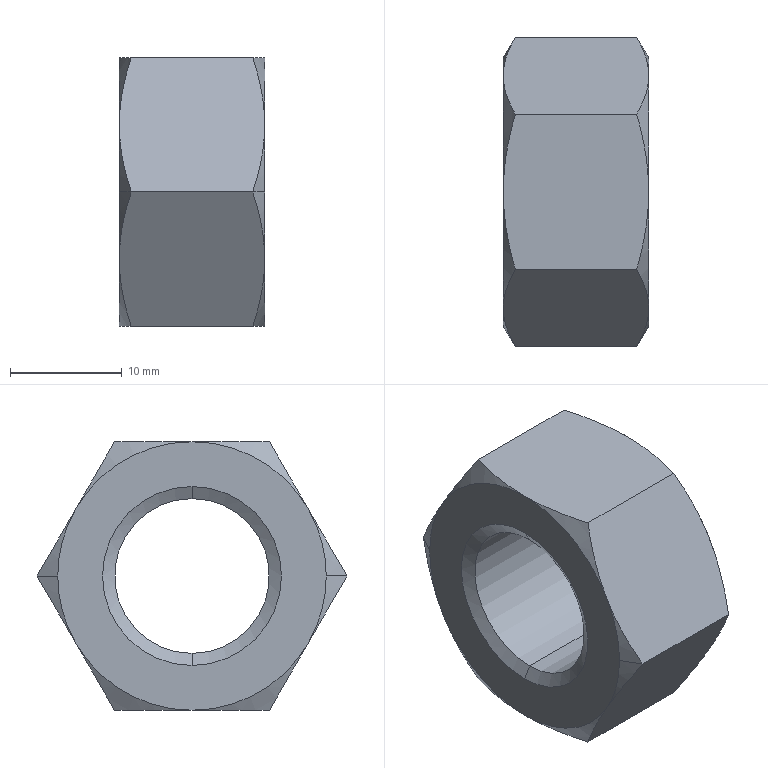Part | STEP file | KS B 1012 - M 16 | 1 solid | 30 faces | box 13 x 27.713 x 24 mm | volume 4470 mm3 | cone 20 | plane 8 | cylinder 2 | commonest cylinder face diameters 13.835 x2